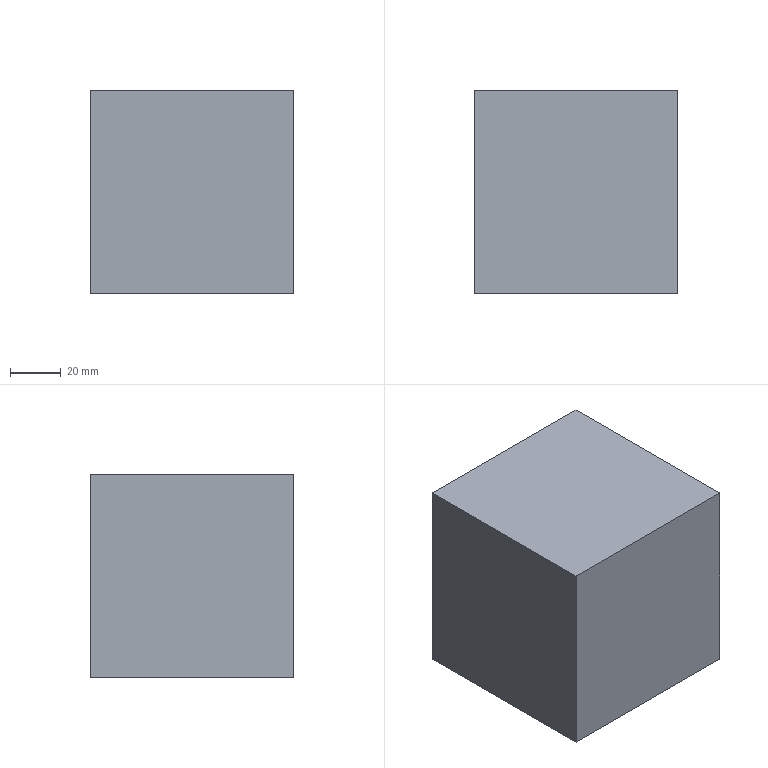Part | SolidWorks | features Extrusion 1 | 1 solid | 6 faces | box 80 x 80 x 80 mm | volume 512000 mm3 | plane 6
STEP:
#1=CARTESIAN_POINT('',(-40.,40.,0.));
#2=VERTEX_POINT('',#1);
#3=CARTESIAN_POINT('',(-40.,-40.,0.));
#4=VERTEX_POINT('',#3);
#5=CARTESIAN_POINT('',(-40.,-40.,0.));
#6=DIRECTION('',(0.,-1.,0.));
#7=VECTOR('',#6,1000.);
#8=LINE('',#5,#7);
#9=EDGE_CURVE('',#2,#4,#8,.T.);
#10=ORIENTED_EDGE('',*,*,#9,.T.);
#11=CARTESIAN_POINT('',(-40.,-40.,80.));
#12=VERTEX_POINT('',#11);
#13=CARTESIAN_POINT('',(-40.,-40.,80.));
#14=DIRECTION('',(0.,0.,-1.));
#15=VECTOR('',#14,1000.);
#16=LINE('',#13,#15);
#17=EDGE_CURVE('',#12,#4,#16,.T.);
#18=ORIENTED_EDGE('',*,*,#17,.F.);
#19=CARTESIAN_POINT('',(-40.,40.,80.));
#20=VERTEX_POINT('',#19);
#21=CARTESIAN_POINT('',(-40.,-40.,80.));
#22=DIRECTION('',(0.,-1.,0.));
#23=VECTOR('',#22,1000.);
#24=LINE('',#21,#23);
#25=EDGE_CURVE('',#20,#12,#24,.T.);
#26=ORIENTED_EDGE('',*,*,#25,.F.);
#27=CARTESIAN_POINT('',(-40.,40.,80.));
#28=DIRECTION('',(0.,0.,-1.));
#29=VECTOR('',#28,1000.);
#30=LINE('',#27,#29);
#31=EDGE_CURVE('',#20,#2,#30,.T.);
#32=ORIENTED_EDGE('',*,*,#31,.T.);
#33=EDGE_LOOP('',(#10,#18,#26,#32));
#34=FACE_OUTER_BOUND('',#33,.T.);
#35=CARTESIAN_POINT('',(-40.,-40.,80.));
#36=DIRECTION('',(1.,0.,0.));
#37=DIRECTION('',(0.,0.,-1.));
#38=AXIS2_PLACEMENT_3D('',#35,#36,#37);
#39=PLANE('',#38);
#40=ADVANCED_FACE('',(#34),#39,.F.);
#41=CARTESIAN_POINT('',(40.,-40.,0.));
#42=VERTEX_POINT('',#41);
#43=CARTESIAN_POINT('',(40.,-40.,0.));
#44=DIRECTION('',(1.,0.,0.));
#45=VECTOR('',#44,1000.);
#46=LINE('',#43,#45);
#47=EDGE_CURVE('',#4,#42,#46,.T.);
#48=ORIENTED_EDGE('',*,*,#47,.T.);
#49=CARTESIAN_POINT('',(40.,-40.,80.));
#50=VERTEX_POINT('',#49);
#51=CARTESIAN_POINT('',(40.,-40.,80.));
#52=DIRECTION('',(0.,0.,-1.));
#53=VECTOR('',#52,1000.);
#54=LINE('',#51,#53);
#55=EDGE_CURVE('',#50,#42,#54,.T.);
#56=ORIENTED_EDGE('',*,*,#55,.F.);
#57=CARTESIAN_POINT('',(40.,-40.,80.));
#58=DIRECTION('',(1.,0.,0.));
#59=VECTOR('',#58,1000.);
#60=LINE('',#57,#59);
#61=EDGE_CURVE('',#12,#50,#60,.T.);
#62=ORIENTED_EDGE('',*,*,#61,.F.);
#63=ORIENTED_EDGE('',*,*,#17,.T.);
#64=EDGE_LOOP('',(#48,#56,#62,#63));
#65=FACE_OUTER_BOUND('',#64,.T.);
#66=CARTESIAN_POINT('',(40.,-40.,80.));
#67=DIRECTION('',(0.,1.,0.));
#68=DIRECTION('',(-1.,0.,0.));
#69=AXIS2_PLACEMENT_3D('',#66,#67,#68);
#70=PLANE('',#69);
#71=ADVANCED_FACE('',(#65),#70,.F.);
#72=CARTESIAN_POINT('',(40.,40.,0.));
#73=VERTEX_POINT('',#72);
#74=CARTESIAN_POINT('',(40.,-40.,0.));
#75=DIRECTION('',(0.,1.,0.));
#76=VECTOR('',#75,1000.);
#77=LINE('',#74,#76);
#78=EDGE_CURVE('',#42,#73,#77,.T.);
#79=ORIENTED_EDGE('',*,*,#78,.T.);
#80=CARTESIAN_POINT('',(40.,40.,80.));
#81=VERTEX_POINT('',#80);
#82=CARTESIAN_POINT('',(40.,40.,80.));
#83=DIRECTION('',(0.,0.,-1.));
#84=VECTOR('',#83,1000.);
#85=LINE('',#82,#84);
#86=EDGE_CURVE('',#81,#73,#85,.T.);
#87=ORIENTED_EDGE('',*,*,#86,.F.);
#88=CARTESIAN_POINT('',(40.,-40.,80.));
#89=DIRECTION('',(0.,1.,0.));
#90=VECTOR('',#89,1000.);
#91=LINE('',#88,#90);
#92=EDGE_CURVE('',#50,#81,#91,.T.);
#93=ORIENTED_EDGE('',*,*,#92,.F.);
#94=ORIENTED_EDGE('',*,*,#55,.T.);
#95=EDGE_LOOP('',(#79,#87,#93,#94));
#96=FACE_OUTER_BOUND('',#95,.T.);
#97=CARTESIAN_POINT('',(40.,-40.,80.));
#98=DIRECTION('',(-1.,0.,0.));
#99=DIRECTION('',(0.,0.,1.));
#100=AXIS2_PLACEMENT_3D('',#97,#98,#99);
#101=PLANE('',#100);
#102=ADVANCED_FACE('',(#96),#101,.F.);
#103=CARTESIAN_POINT('',(40.,40.,0.));
#104=DIRECTION('',(-1.,0.,0.));
#105=VECTOR('',#104,1000.);
#106=LINE('',#103,#105);
#107=EDGE_CURVE('',#73,#2,#106,.T.);
#108=ORIENTED_EDGE('',*,*,#107,.T.);
#109=ORIENTED_EDGE('',*,*,#31,.F.);
#110=CARTESIAN_POINT('',(40.,40.,80.));
#111=DIRECTION('',(-1.,0.,0.));
#112=VECTOR('',#111,1000.);
#113=LINE('',#110,#112);
#114=EDGE_CURVE('',#81,#20,#113,.T.);
#115=ORIENTED_EDGE('',*,*,#114,.F.);
#116=ORIENTED_EDGE('',*,*,#86,.T.);
#117=EDGE_LOOP('',(#108,#109,#115,#116));
#118=FACE_OUTER_BOUND('',#117,.T.);
#119=CARTESIAN_POINT('',(40.,40.,80.));
#120=DIRECTION('',(0.,-1.,0.));
#121=DIRECTION('',(1.,0.,0.));
#122=AXIS2_PLACEMENT_3D('',#119,#120,#121);
#123=PLANE('',#122);
#124=ADVANCED_FACE('',(#118),#123,.F.);
#125=ORIENTED_EDGE('',*,*,#25,.T.);
#126=ORIENTED_EDGE('',*,*,#61,.T.);
#127=ORIENTED_EDGE('',*,*,#92,.T.);
#128=ORIENTED_EDGE('',*,*,#114,.T.);
#129=EDGE_LOOP('',(#125,#126,#127,#128));
#130=FACE_OUTER_BOUND('',#129,.T.);
#131=CARTESIAN_POINT('',(0.,0.,80.));
#132=DIRECTION('',(0.,0.,1.));
#133=DIRECTION('',(1.,0.,0.));
#134=AXIS2_PLACEMENT_3D('',#131,#132,#133);
#135=PLANE('',#134);
#136=ADVANCED_FACE('',(#130),#135,.T.);
#137=ORIENTED_EDGE('',*,*,#9,.F.);
#138=ORIENTED_EDGE('',*,*,#107,.F.);
#139=ORIENTED_EDGE('',*,*,#78,.F.);
#140=ORIENTED_EDGE('',*,*,#47,.F.);
#141=EDGE_LOOP('',(#137,#138,#139,#140));
#142=FACE_OUTER_BOUND('',#141,.T.);
#143=CARTESIAN_POINT('',(0.,0.,0.));
#144=DIRECTION('',(0.,0.,1.));
#145=DIRECTION('',(1.,0.,0.));
#146=AXIS2_PLACEMENT_3D('',#143,#144,#145);
#147=PLANE('',#146);
#148=ADVANCED_FACE('',(#142),#147,.F.);
#149=CLOSED_SHELL('',(#40,#71,#102,#124,#136,#148));
#150=MANIFOLD_SOLID_BREP('',#149);
#151=CARTESIAN_POINT('',(0.,0.,0.));
#152=DIRECTION('',(0.,0.,1.));
#153=DIRECTION('',(1.,0.,0.));
#154=AXIS2_PLACEMENT_3D('',#151,#152,#153);
#155=(LENGTH_UNIT()NAMED_UNIT(*)SI_UNIT(.MILLI.,.METRE.));
#156=UNCERTAINTY_MEASURE_WITH_UNIT(LENGTH_MEASURE(0.00001),#155,'','');
#157=(NAMED_UNIT(*)PLANE_ANGLE_UNIT()SI_UNIT($,.RADIAN.));
#158=(NAMED_UNIT(*)SI_UNIT($,.STERADIAN.)SOLID_ANGLE_UNIT());
#159=(GEOMETRIC_REPRESENTATION_CONTEXT(3)GLOBAL_UNCERTAINTY_ASSIGNED_CONTEXT((#156))GLOBAL_UNIT_ASSIGNED_CONTEXT((#155,#157,#158))REPRESENTATION_CONTEXT('',''));
#160=ADVANCED_BREP_SHAPE_REPRESENTATION('',(#150,#154),#159);